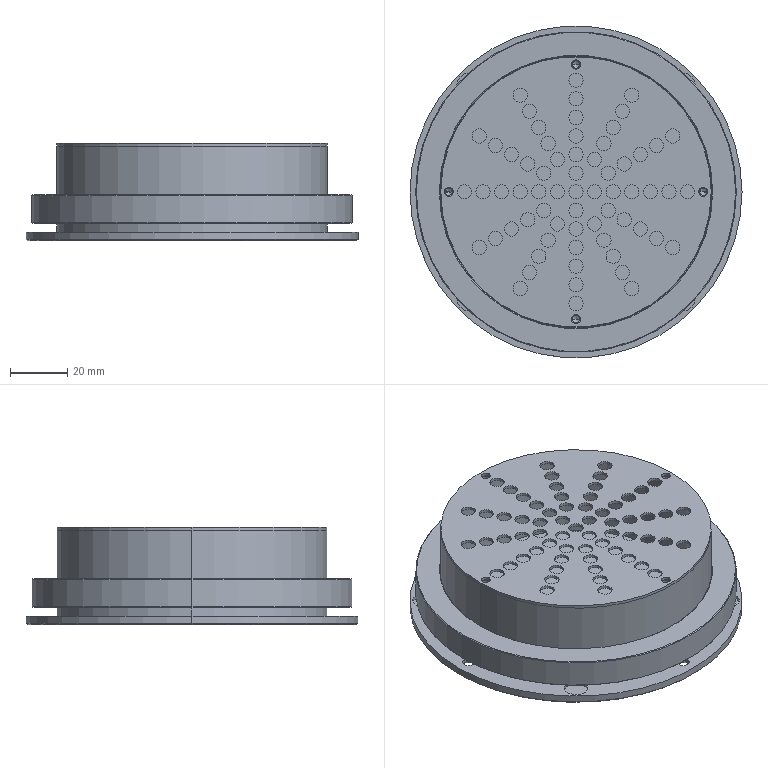Part | SolidWorks | features InContextFeatHolder 2, RefAxis 1 | 3 solids | 242 faces | box 116 x 116 x 34 mm | volume 105330 mm3 | cylinder 194 | cone 26 | plane 22 | commonest cylinder face diameters 5 x130 3.3 x16 2.5 x8 3.2 x8 4.2 x8 8.2 x8